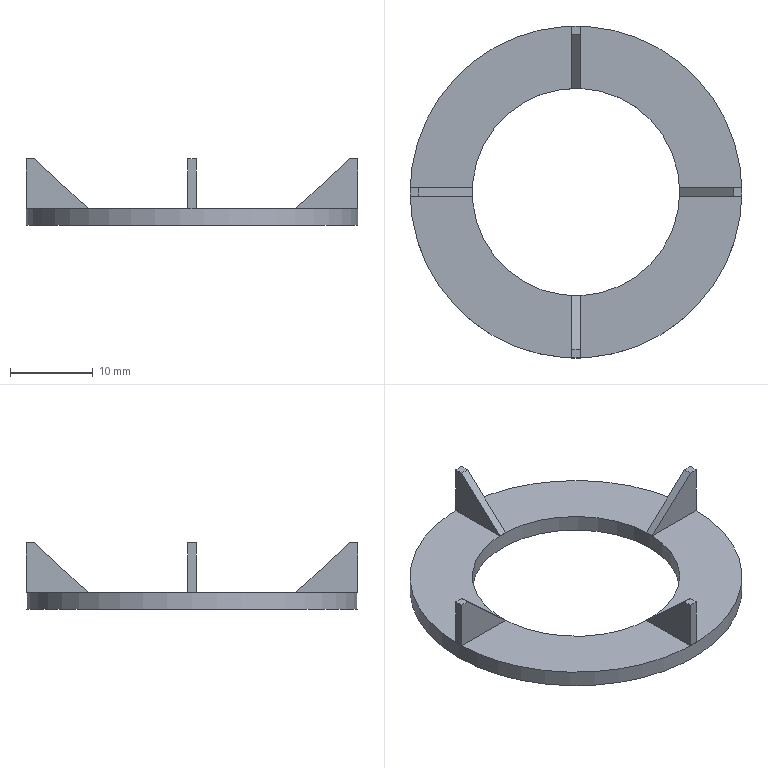Part | NX | features EXTRUDE 5, EXTRACT_STRING 4, DATUM_CSYS 3, Instance Feature 3, SKETCH 2, Pattern Feature 1 | 5 solids | 28 faces | box 40 x 40 x 8 mm | volume 1634 mm3 | plane 26 | cylinder 2 | commonest cylinder face diameters 25 x1 40 x1
STEP:
#1=CARTESIAN_POINT('',(20.,-0.5,8.));
#2=VERTEX_POINT('',#1);
#3=CARTESIAN_POINT('',(20.,-0.5,2.));
#4=VERTEX_POINT('',#3);
#5=CARTESIAN_POINT('',(20.,-0.5,8.));
#6=DIRECTION('',(0.,0.,-1.));
#7=VECTOR('',#6,1000.);
#8=LINE('',#5,#7);
#9=EDGE_CURVE('',#2,#4,#8,.T.);
#10=ORIENTED_EDGE('',*,*,#9,.T.);
#11=CARTESIAN_POINT('',(20.,0.5,2.));
#12=VERTEX_POINT('',#11);
#13=CARTESIAN_POINT('',(20.,0.5,2.));
#14=DIRECTION('',(0.,-1.,0.));
#15=VECTOR('',#14,1000.);
#16=LINE('',#13,#15);
#17=EDGE_CURVE('',#12,#4,#16,.T.);
#18=ORIENTED_EDGE('',*,*,#17,.F.);
#19=CARTESIAN_POINT('',(20.,0.5,8.));
#20=VERTEX_POINT('',#19);
#21=CARTESIAN_POINT('',(20.,0.5,8.));
#22=DIRECTION('',(0.,0.,-1.));
#23=VECTOR('',#22,1000.);
#24=LINE('',#21,#23);
#25=EDGE_CURVE('',#20,#12,#24,.T.);
#26=ORIENTED_EDGE('',*,*,#25,.F.);
#27=CARTESIAN_POINT('',(20.,0.5,8.));
#28=DIRECTION('',(0.,-1.,0.));
#29=VECTOR('',#28,1000.);
#30=LINE('',#27,#29);
#31=EDGE_CURVE('',#20,#2,#30,.T.);
#32=ORIENTED_EDGE('',*,*,#31,.T.);
#33=EDGE_LOOP('',(#10,#18,#26,#32));
#34=FACE_BOUND('',#33,.T.);
#35=CARTESIAN_POINT('',(20.,0.5,8.));
#36=DIRECTION('',(-1.,0.,0.));
#37=DIRECTION('',(0.,-1.,0.));
#38=AXIS2_PLACEMENT_3D('',#35,#36,#37);
#39=PLANE('',#38);
#40=ADVANCED_FACE('',(#34),#39,.F.);
#41=CARTESIAN_POINT('',(12.5,-0.5,2.));
#42=VERTEX_POINT('',#41);
#43=CARTESIAN_POINT('',(20.,-0.5,2.));
#44=DIRECTION('',(-1.,0.,0.));
#45=VECTOR('',#44,1000.);
#46=LINE('',#43,#45);
#47=EDGE_CURVE('',#4,#42,#46,.T.);
#48=ORIENTED_EDGE('',*,*,#47,.T.);
#49=CARTESIAN_POINT('',(12.5,0.5,2.));
#50=VERTEX_POINT('',#49);
#51=CARTESIAN_POINT('',(12.5,0.5,2.));
#52=DIRECTION('',(0.,-1.,0.));
#53=VECTOR('',#52,1000.);
#54=LINE('',#51,#53);
#55=EDGE_CURVE('',#50,#42,#54,.T.);
#56=ORIENTED_EDGE('',*,*,#55,.F.);
#57=CARTESIAN_POINT('',(20.,0.5,2.));
#58=DIRECTION('',(-1.,0.,0.));
#59=VECTOR('',#58,1000.);
#60=LINE('',#57,#59);
#61=EDGE_CURVE('',#12,#50,#60,.T.);
#62=ORIENTED_EDGE('',*,*,#61,.F.);
#63=ORIENTED_EDGE('',*,*,#17,.T.);
#64=EDGE_LOOP('',(#48,#56,#62,#63));
#65=FACE_BOUND('',#64,.T.);
#66=CARTESIAN_POINT('',(20.,0.5,2.));
#67=DIRECTION('',(0.,0.,1.));
#68=DIRECTION('',(1.,0.,0.));
#69=AXIS2_PLACEMENT_3D('',#66,#67,#68);
#70=PLANE('',#69);
#71=ADVANCED_FACE('',(#65),#70,.F.);
#72=CARTESIAN_POINT('',(19.,-0.5,8.));
#73=VERTEX_POINT('',#72);
#74=CARTESIAN_POINT('',(12.5,-0.5,2.));
#75=DIRECTION('',(0.7348,0.,0.6783));
#76=VECTOR('',#75,1000.);
#77=LINE('',#74,#76);
#78=EDGE_CURVE('',#42,#73,#77,.T.);
#79=ORIENTED_EDGE('',*,*,#78,.T.);
#80=CARTESIAN_POINT('',(19.,0.5,8.));
#81=VERTEX_POINT('',#80);
#82=CARTESIAN_POINT('',(19.,0.5,8.));
#83=DIRECTION('',(0.,-1.,0.));
#84=VECTOR('',#83,1000.);
#85=LINE('',#82,#84);
#86=EDGE_CURVE('',#81,#73,#85,.T.);
#87=ORIENTED_EDGE('',*,*,#86,.F.);
#88=CARTESIAN_POINT('',(12.5,0.5,2.));
#89=DIRECTION('',(0.7348,0.,0.6783));
#90=VECTOR('',#89,1000.);
#91=LINE('',#88,#90);
#92=EDGE_CURVE('',#50,#81,#91,.T.);
#93=ORIENTED_EDGE('',*,*,#92,.F.);
#94=ORIENTED_EDGE('',*,*,#55,.T.);
#95=EDGE_LOOP('',(#79,#87,#93,#94));
#96=FACE_BOUND('',#95,.T.);
#97=CARTESIAN_POINT('',(12.5,0.5,2.));
#98=DIRECTION('',(0.6783,0.,-0.7348));
#99=DIRECTION('',(-0.7348,0.,-0.6783));
#100=AXIS2_PLACEMENT_3D('',#97,#98,#99);
#101=PLANE('',#100);
#102=ADVANCED_FACE('',(#96),#101,.F.);
#103=CARTESIAN_POINT('',(19.,-0.5,8.));
#104=DIRECTION('',(1.,0.,0.));
#105=VECTOR('',#104,1000.);
#106=LINE('',#103,#105);
#107=EDGE_CURVE('',#73,#2,#106,.T.);
#108=ORIENTED_EDGE('',*,*,#107,.T.);
#109=ORIENTED_EDGE('',*,*,#31,.F.);
#110=CARTESIAN_POINT('',(19.,0.5,8.));
#111=DIRECTION('',(1.,0.,0.));
#112=VECTOR('',#111,1000.);
#113=LINE('',#110,#112);
#114=EDGE_CURVE('',#81,#20,#113,.T.);
#115=ORIENTED_EDGE('',*,*,#114,.F.);
#116=ORIENTED_EDGE('',*,*,#86,.T.);
#117=EDGE_LOOP('',(#108,#109,#115,#116));
#118=FACE_BOUND('',#117,.T.);
#119=CARTESIAN_POINT('',(19.,0.5,8.));
#120=DIRECTION('',(0.,0.,-1.));
#121=DIRECTION('',(-1.,0.,0.));
#122=AXIS2_PLACEMENT_3D('',#119,#120,#121);
#123=PLANE('',#122);
#124=ADVANCED_FACE('',(#118),#123,.F.);
#125=ORIENTED_EDGE('',*,*,#25,.T.);
#126=ORIENTED_EDGE('',*,*,#61,.T.);
#127=ORIENTED_EDGE('',*,*,#92,.T.);
#128=ORIENTED_EDGE('',*,*,#114,.T.);
#129=EDGE_LOOP('',(#125,#126,#127,#128));
#130=FACE_BOUND('',#129,.T.);
#131=CARTESIAN_POINT('',(0.,0.5,0.));
#132=DIRECTION('',(0.,1.,0.));
#133=DIRECTION('',(-1.,0.,0.));
#134=AXIS2_PLACEMENT_3D('',#131,#132,#133);
#135=PLANE('',#134);
#136=ADVANCED_FACE('',(#130),#135,.T.);
#137=ORIENTED_EDGE('',*,*,#9,.F.);
#138=ORIENTED_EDGE('',*,*,#107,.F.);
#139=ORIENTED_EDGE('',*,*,#78,.F.);
#140=ORIENTED_EDGE('',*,*,#47,.F.);
#141=EDGE_LOOP('',(#137,#138,#139,#140));
#142=FACE_BOUND('',#141,.T.);
#143=CARTESIAN_POINT('',(0.,-0.5,0.));
#144=DIRECTION('',(0.,1.,0.));
#145=DIRECTION('',(-1.,0.,0.));
#146=AXIS2_PLACEMENT_3D('',#143,#144,#145);
#147=PLANE('',#146);
#148=ADVANCED_FACE('',(#142),#147,.F.);
#149=CLOSED_SHELL('',(#40,#71,#102,#124,#136,#148));
#150=MANIFOLD_SOLID_BREP('',#149);
#151=CARTESIAN_POINT('',(-20.,0.5,8.));
#152=VERTEX_POINT('',#151);
#153=CARTESIAN_POINT('',(-20.,0.5,2.));
#154=VERTEX_POINT('',#153);
#155=CARTESIAN_POINT('',(-20.,0.5,8.));
#156=DIRECTION('',(0.,0.,-1.));
#157=VECTOR('',#156,1000.);
#158=LINE('',#155,#157);
#159=EDGE_CURVE('',#152,#154,#158,.T.);
#160=ORIENTED_EDGE('',*,*,#159,.T.);
#161=CARTESIAN_POINT('',(-20.,-0.5,2.));
#162=VERTEX_POINT('',#161);
#163=CARTESIAN_POINT('',(-20.,-0.5,2.));
#164=DIRECTION('',(0.,1.,0.));
#165=VECTOR('',#164,1000.);
#166=LINE('',#163,#165);
#167=EDGE_CURVE('',#162,#154,#166,.T.);
#168=ORIENTED_EDGE('',*,*,#167,.F.);
#169=CARTESIAN_POINT('',(-20.,-0.5,8.));
#170=VERTEX_POINT('',#169);
#171=CARTESIAN_POINT('',(-20.,-0.5,8.));
#172=DIRECTION('',(0.,0.,-1.));
#173=VECTOR('',#172,1000.);
#174=LINE('',#171,#173);
#175=EDGE_CURVE('',#170,#162,#174,.T.);
#176=ORIENTED_EDGE('',*,*,#175,.F.);
#177=CARTESIAN_POINT('',(-20.,-0.5,8.));
#178=DIRECTION('',(0.,1.,0.));
#179=VECTOR('',#178,1000.);
#180=LINE('',#177,#179);
#181=EDGE_CURVE('',#170,#152,#180,.T.);
#182=ORIENTED_EDGE('',*,*,#181,.T.);
#183=EDGE_LOOP('',(#160,#168,#176,#182));
#184=FACE_BOUND('',#183,.T.);
#185=CARTESIAN_POINT('',(-20.,-0.5,8.));
#186=DIRECTION('',(1.,0.,0.));
#187=DIRECTION('',(0.,1.,0.));
#188=AXIS2_PLACEMENT_3D('',#185,#186,#187);
#189=PLANE('',#188);
#190=ADVANCED_FACE('',(#184),#189,.F.);
#191=CARTESIAN_POINT('',(-12.5,0.5,2.));
#192=VERTEX_POINT('',#191);
#193=CARTESIAN_POINT('',(-20.,0.5,2.));
#194=DIRECTION('',(1.,0.,0.));
#195=VECTOR('',#194,1000.);
#196=LINE('',#193,#195);
#197=EDGE_CURVE('',#154,#192,#196,.T.);
#198=ORIENTED_EDGE('',*,*,#197,.T.);
#199=CARTESIAN_POINT('',(-12.5,-0.5,2.));
#200=VERTEX_POINT('',#199);
#201=CARTESIAN_POINT('',(-12.5,-0.5,2.));
#202=DIRECTION('',(0.,1.,0.));
#203=VECTOR('',#202,1000.);
#204=LINE('',#201,#203);
#205=EDGE_CURVE('',#200,#192,#204,.T.);
#206=ORIENTED_EDGE('',*,*,#205,.F.);
#207=CARTESIAN_POINT('',(-20.,-0.5,2.));
#208=DIRECTION('',(1.,0.,0.));
#209=VECTOR('',#208,1000.);
#210=LINE('',#207,#209);
#211=EDGE_CURVE('',#162,#200,#210,.T.);
#212=ORIENTED_EDGE('',*,*,#211,.F.);
#213=ORIENTED_EDGE('',*,*,#167,.T.);
#214=EDGE_LOOP('',(#198,#206,#212,#213));
#215=FACE_BOUND('',#214,.T.);
#216=CARTESIAN_POINT('',(-20.,-0.5,2.));
#217=DIRECTION('',(0.,0.,1.));
#218=DIRECTION('',(1.,0.,0.));
#219=AXIS2_PLACEMENT_3D('',#216,#217,#218);
#220=PLANE('',#219);
#221=ADVANCED_FACE('',(#215),#220,.F.);
#222=CARTESIAN_POINT('',(-19.,0.5,8.));
#223=VERTEX_POINT('',#222);
#224=CARTESIAN_POINT('',(-12.5,0.5,2.));
#225=DIRECTION('',(-0.7348,0.,0.6783));
#226=VECTOR('',#225,1000.);
#227=LINE('',#224,#226);
#228=EDGE_CURVE('',#192,#223,#227,.T.);
#229=ORIENTED_EDGE('',*,*,#228,.T.);
#230=CARTESIAN_POINT('',(-19.,-0.5,8.));
#231=VERTEX_POINT('',#230);
#232=CARTESIAN_POINT('',(-19.,-0.5,8.));
#233=DIRECTION('',(0.,1.,0.));
#234=VECTOR('',#233,1000.);
#235=LINE('',#232,#234);
#236=EDGE_CURVE('',#231,#223,#235,.T.);
#237=ORIENTED_EDGE('',*,*,#236,.F.);
#238=CARTESIAN_POINT('',(-12.5,-0.5,2.));
#239=DIRECTION('',(-0.7348,0.,0.6783));
#240=VECTOR('',#239,1000.);
#241=LINE('',#238,#240);
#242=EDGE_CURVE('',#200,#231,#241,.T.);
#243=ORIENTED_EDGE('',*,*,#242,.F.);
#244=ORIENTED_EDGE('',*,*,#205,.T.);
#245=EDGE_LOOP('',(#229,#237,#243,#244));
#246=FACE_BOUND('',#245,.T.);
#247=CARTESIAN_POINT('',(-12.5,-0.5,2.));
#248=DIRECTION('',(-0.6783,0.,-0.7348));
#249=DIRECTION('',(-0.7348,0.,0.6783));
#250=AXIS2_PLACEMENT_3D('',#247,#248,#249);
#251=PLANE('',#250);
#252=ADVANCED_FACE('',(#246),#251,.F.);
#253=CARTESIAN_POINT('',(-19.,0.5,8.));
#254=DIRECTION('',(-1.,0.,0.));
#255=VECTOR('',#254,1000.);
#256=LINE('',#253,#255);
#257=EDGE_CURVE('',#223,#152,#256,.T.);
#258=ORIENTED_EDGE('',*,*,#257,.T.);
#259=ORIENTED_EDGE('',*,*,#181,.F.);
#260=CARTESIAN_POINT('',(-19.,-0.5,8.));
#261=DIRECTION('',(-1.,0.,0.));
#262=VECTOR('',#261,1000.);
#263=LINE('',#260,#262);
#264=EDGE_CURVE('',#231,#170,#263,.T.);
#265=ORIENTED_EDGE('',*,*,#264,.F.);
#266=ORIENTED_EDGE('',*,*,#236,.T.);
#267=EDGE_LOOP('',(#258,#259,#265,#266));
#268=FACE_BOUND('',#267,.T.);
#269=CARTESIAN_POINT('',(-19.,-0.5,8.));
#270=DIRECTION('',(0.,0.,-1.));
#271=DIRECTION('',(-1.,0.,0.));
#272=AXIS2_PLACEMENT_3D('',#269,#270,#271);
#273=PLANE('',#272);
#274=ADVANCED_FACE('',(#268),#273,.F.);
#275=ORIENTED_EDGE('',*,*,#175,.T.);
#276=ORIENTED_EDGE('',*,*,#211,.T.);
#277=ORIENTED_EDGE('',*,*,#242,.T.);
#278=ORIENTED_EDGE('',*,*,#264,.T.);
#279=EDGE_LOOP('',(#275,#276,#277,#278));
#280=FACE_BOUND('',#279,.T.);
#281=CARTESIAN_POINT('',(0.,-0.5,0.));
#282=DIRECTION('',(0.,-1.,0.));
#283=DIRECTION('',(1.,0.,0.));
#284=AXIS2_PLACEMENT_3D('',#281,#282,#283);
#285=PLANE('',#284);
#286=ADVANCED_FACE('',(#280),#285,.T.);
#287=ORIENTED_EDGE('',*,*,#159,.F.);
#288=ORIENTED_EDGE('',*,*,#257,.F.);
#289=ORIENTED_EDGE('',*,*,#228,.F.);
#290=ORIENTED_EDGE('',*,*,#197,.F.);
#291=EDGE_LOOP('',(#287,#288,#289,#290));
#292=FACE_BOUND('',#291,.T.);
#293=CARTESIAN_POINT('',(0.,0.5,0.));
#294=DIRECTION('',(0.,-1.,0.));
#295=DIRECTION('',(1.,0.,0.));
#296=AXIS2_PLACEMENT_3D('',#293,#294,#295);
#297=PLANE('',#296);
#298=ADVANCED_FACE('',(#292),#297,.F.);
#299=CLOSED_SHELL('',(#190,#221,#252,#274,#286,#298));
#300=MANIFOLD_SOLID_BREP('',#299);
#301=CARTESIAN_POINT('',(20.,0.,0.));
#302=VERTEX_POINT('',#301);
#303=CARTESIAN_POINT('',(0.,0.,0.));
#304=DIRECTION('',(0.,0.,1.));
#305=DIRECTION('',(1.,0.,0.));
#306=AXIS2_PLACEMENT_3D('',#303,#304,#305);
#307=CIRCLE('',#306,20.);
#308=EDGE_CURVE('',#302,#302,#307,.T.);
#309=ORIENTED_EDGE('',*,*,#308,.T.);
#310=EDGE_LOOP('',(#309));
#311=FACE_BOUND('',#310,.T.);
#312=CARTESIAN_POINT('',(20.,0.,2.));
#313=VERTEX_POINT('',#312);
#314=CARTESIAN_POINT('',(0.,0.,2.));
#315=DIRECTION('',(0.,0.,1.));
#316=DIRECTION('',(1.,0.,0.));
#317=AXIS2_PLACEMENT_3D('',#314,#315,#316);
#318=CIRCLE('',#317,20.);
#319=EDGE_CURVE('',#313,#313,#318,.T.);
#320=ORIENTED_EDGE('',*,*,#319,.F.);
#321=EDGE_LOOP('',(#320));
#322=FACE_BOUND('',#321,.T.);
#323=CARTESIAN_POINT('',(0.,0.,0.));
#324=DIRECTION('',(0.,0.,1.));
#325=DIRECTION('',(1.,0.,0.));
#326=AXIS2_PLACEMENT_3D('',#323,#324,#325);
#327=CYLINDRICAL_SURFACE('',#326,20.);
#328=ADVANCED_FACE('',(#311,#322),#327,.T.);
#329=CARTESIAN_POINT('',(12.5,0.,0.));
#330=VERTEX_POINT('',#329);
#331=CARTESIAN_POINT('',(0.,0.,0.));
#332=DIRECTION('',(0.,0.,1.));
#333=DIRECTION('',(1.,0.,0.));
#334=AXIS2_PLACEMENT_3D('',#331,#332,#333);
#335=CIRCLE('',#334,12.5);
#336=EDGE_CURVE('',#330,#330,#335,.T.);
#337=ORIENTED_EDGE('',*,*,#336,.F.);
#338=EDGE_LOOP('',(#337));
#339=FACE_BOUND('',#338,.T.);
#340=CARTESIAN_POINT('',(12.5,0.,2.));
#341=VERTEX_POINT('',#340);
#342=CARTESIAN_POINT('',(0.,0.,2.));
#343=DIRECTION('',(0.,0.,1.));
#344=DIRECTION('',(1.,0.,0.));
#345=AXIS2_PLACEMENT_3D('',#342,#343,#344);
#346=CIRCLE('',#345,12.5);
#347=EDGE_CURVE('',#341,#341,#346,.T.);
#348=ORIENTED_EDGE('',*,*,#347,.T.);
#349=EDGE_LOOP('',(#348));
#350=FACE_BOUND('',#349,.T.);
#351=CARTESIAN_POINT('',(0.,0.,0.));
#352=DIRECTION('',(0.,0.,1.));
#353=DIRECTION('',(1.,0.,0.));
#354=AXIS2_PLACEMENT_3D('',#351,#352,#353);
#355=CYLINDRICAL_SURFACE('',#354,12.5);
#356=ADVANCED_FACE('',(#339,#350),#355,.F.);
#357=ORIENTED_EDGE('',*,*,#308,.F.);
#358=EDGE_LOOP('',(#357));
#359=FACE_BOUND('',#358,.T.);
#360=ORIENTED_EDGE('',*,*,#336,.T.);
#361=EDGE_LOOP('',(#360));
#362=FACE_BOUND('',#361,.T.);
#363=CARTESIAN_POINT('',(0.,0.,0.));
#364=DIRECTION('',(0.,0.,1.));
#365=DIRECTION('',(1.,0.,0.));
#366=AXIS2_PLACEMENT_3D('',#363,#364,#365);
#367=PLANE('',#366);
#368=ADVANCED_FACE('',(#359,#362),#367,.F.);
#369=ORIENTED_EDGE('',*,*,#319,.T.);
#370=EDGE_LOOP('',(#369));
#371=FACE_BOUND('',#370,.T.);
#372=ORIENTED_EDGE('',*,*,#347,.F.);
#373=EDGE_LOOP('',(#372));
#374=FACE_BOUND('',#373,.T.);
#375=CARTESIAN_POINT('',(0.,0.,2.));
#376=DIRECTION('',(0.,0.,1.));
#377=DIRECTION('',(1.,0.,0.));
#378=AXIS2_PLACEMENT_3D('',#375,#376,#377);
#379=PLANE('',#378);
#380=ADVANCED_FACE('',(#371,#374),#379,.T.);
#381=CLOSED_SHELL('',(#328,#356,#368,#380));
#382=MANIFOLD_SOLID_BREP('',#381);
#383=CARTESIAN_POINT('',(0.5,20.,8.));
#384=VERTEX_POINT('',#383);
#385=CARTESIAN_POINT('',(0.5,20.,2.));
#386=VERTEX_POINT('',#385);
#387=CARTESIAN_POINT('',(0.5,20.,8.));
#388=DIRECTION('',(0.,0.,-1.));
#389=VECTOR('',#388,1000.);
#390=LINE('',#387,#389);
#391=EDGE_CURVE('',#384,#386,#390,.T.);
#392=ORIENTED_EDGE('',*,*,#391,.T.);
#393=CARTESIAN_POINT('',(-0.5,20.,2.));
#394=VERTEX_POINT('',#393);
#395=CARTESIAN_POINT('',(-0.5,20.,2.));
#396=DIRECTION('',(1.,0.,0.));
#397=VECTOR('',#396,1000.);
#398=LINE('',#395,#397);
#399=EDGE_CURVE('',#394,#386,#398,.T.);
#400=ORIENTED_EDGE('',*,*,#399,.F.);
#401=CARTESIAN_POINT('',(-0.5,20.,8.));
#402=VERTEX_POINT('',#401);
#403=CARTESIAN_POINT('',(-0.5,20.,8.));
#404=DIRECTION('',(0.,0.,-1.));
#405=VECTOR('',#404,1000.);
#406=LINE('',#403,#405);
#407=EDGE_CURVE('',#402,#394,#406,.T.);
#408=ORIENTED_EDGE('',*,*,#407,.F.);
#409=CARTESIAN_POINT('',(-0.5,20.,8.));
#410=DIRECTION('',(1.,0.,0.));
#411=VECTOR('',#410,1000.);
#412=LINE('',#409,#411);
#413=EDGE_CURVE('',#402,#384,#412,.T.);
#414=ORIENTED_EDGE('',*,*,#413,.T.);
#415=EDGE_LOOP('',(#392,#400,#408,#414));
#416=FACE_BOUND('',#415,.T.);
#417=CARTESIAN_POINT('',(-0.5,20.,8.));
#418=DIRECTION('',(0.,-1.,0.));
#419=DIRECTION('',(1.,0.,0.));
#420=AXIS2_PLACEMENT_3D('',#417,#418,#419);
#421=PLANE('',#420);
#422=ADVANCED_FACE('',(#416),#421,.F.);
#423=CARTESIAN_POINT('',(0.5,12.5,2.));
#424=VERTEX_POINT('',#423);
#425=CARTESIAN_POINT('',(0.5,20.,2.));
#426=DIRECTION('',(0.,-1.,0.));
#427=VECTOR('',#426,1000.);
#428=LINE('',#425,#427);
#429=EDGE_CURVE('',#386,#424,#428,.T.);
#430=ORIENTED_EDGE('',*,*,#429,.T.);
#431=CARTESIAN_POINT('',(-0.5,12.5,2.));
#432=VERTEX_POINT('',#431);
#433=CARTESIAN_POINT('',(-0.5,12.5,2.));
#434=DIRECTION('',(1.,0.,0.));
#435=VECTOR('',#434,1000.);
#436=LINE('',#433,#435);
#437=EDGE_CURVE('',#432,#424,#436,.T.);
#438=ORIENTED_EDGE('',*,*,#437,.F.);
#439=CARTESIAN_POINT('',(-0.5,20.,2.));
#440=DIRECTION('',(0.,-1.,0.));
#441=VECTOR('',#440,1000.);
#442=LINE('',#439,#441);
#443=EDGE_CURVE('',#394,#432,#442,.T.);
#444=ORIENTED_EDGE('',*,*,#443,.F.);
#445=ORIENTED_EDGE('',*,*,#399,.T.);
#446=EDGE_LOOP('',(#430,#438,#444,#445));
#447=FACE_BOUND('',#446,.T.);
#448=CARTESIAN_POINT('',(-0.5,20.,2.));
#449=DIRECTION('',(0.,0.,1.));
#450=DIRECTION('',(1.,0.,0.));
#451=AXIS2_PLACEMENT_3D('',#448,#449,#450);
#452=PLANE('',#451);
#453=ADVANCED_FACE('',(#447),#452,.F.);
#454=CARTESIAN_POINT('',(0.5,19.,8.));
#455=VERTEX_POINT('',#454);
#456=CARTESIAN_POINT('',(0.5,12.5,2.));
#457=DIRECTION('',(0.,0.7348,0.6783));
#458=VECTOR('',#457,1000.);
#459=LINE('',#456,#458);
#460=EDGE_CURVE('',#424,#455,#459,.T.);
#461=ORIENTED_EDGE('',*,*,#460,.T.);
#462=CARTESIAN_POINT('',(-0.5,19.,8.));
#463=VERTEX_POINT('',#462);
#464=CARTESIAN_POINT('',(-0.5,19.,8.));
#465=DIRECTION('',(1.,0.,0.));
#466=VECTOR('',#465,1000.);
#467=LINE('',#464,#466);
#468=EDGE_CURVE('',#463,#455,#467,.T.);
#469=ORIENTED_EDGE('',*,*,#468,.F.);
#470=CARTESIAN_POINT('',(-0.5,12.5,2.));
#471=DIRECTION('',(0.,0.7348,0.6783));
#472=VECTOR('',#471,1000.);
#473=LINE('',#470,#472);
#474=EDGE_CURVE('',#432,#463,#473,.T.);
#475=ORIENTED_EDGE('',*,*,#474,.F.);
#476=ORIENTED_EDGE('',*,*,#437,.T.);
#477=EDGE_LOOP('',(#461,#469,#475,#476));
#478=FACE_BOUND('',#477,.T.);
#479=CARTESIAN_POINT('',(-0.5,12.5,2.));
#480=DIRECTION('',(0.,0.6783,-0.7348));
#481=DIRECTION('',(0.,0.7348,0.6783));
#482=AXIS2_PLACEMENT_3D('',#479,#480,#481);
#483=PLANE('',#482);
#484=ADVANCED_FACE('',(#478),#483,.F.);
#485=CARTESIAN_POINT('',(0.5,19.,8.));
#486=DIRECTION('',(0.,1.,0.));
#487=VECTOR('',#486,1000.);
#488=LINE('',#485,#487);
#489=EDGE_CURVE('',#455,#384,#488,.T.);
#490=ORIENTED_EDGE('',*,*,#489,.T.);
#491=ORIENTED_EDGE('',*,*,#413,.F.);
#492=CARTESIAN_POINT('',(-0.5,19.,8.));
#493=DIRECTION('',(0.,1.,0.));
#494=VECTOR('',#493,1000.);
#495=LINE('',#492,#494);
#496=EDGE_CURVE('',#463,#402,#495,.T.);
#497=ORIENTED_EDGE('',*,*,#496,.F.);
#498=ORIENTED_EDGE('',*,*,#468,.T.);
#499=EDGE_LOOP('',(#490,#491,#497,#498));
#500=FACE_BOUND('',#499,.T.);
#501=CARTESIAN_POINT('',(-0.5,19.,8.));
#502=DIRECTION('',(0.,0.,-1.));
#503=DIRECTION('',(-1.,0.,0.));
#504=AXIS2_PLACEMENT_3D('',#501,#502,#503);
#505=PLANE('',#504);
#506=ADVANCED_FACE('',(#500),#505,.F.);
#507=ORIENTED_EDGE('',*,*,#407,.T.);
#508=ORIENTED_EDGE('',*,*,#443,.T.);
#509=ORIENTED_EDGE('',*,*,#474,.T.);
#510=ORIENTED_EDGE('',*,*,#496,.T.);
#511=EDGE_LOOP('',(#507,#508,#509,#510));
#512=FACE_BOUND('',#511,.T.);
#513=CARTESIAN_POINT('',(-0.5,0.,0.));
#514=DIRECTION('',(-1.,0.,0.));
#515=DIRECTION('',(0.,-1.,0.));
#516=AXIS2_PLACEMENT_3D('',#513,#514,#515);
#517=PLANE('',#516);
#518=ADVANCED_FACE('',(#512),#517,.T.);
#519=ORIENTED_EDGE('',*,*,#391,.F.);
#520=ORIENTED_EDGE('',*,*,#489,.F.);
#521=ORIENTED_EDGE('',*,*,#460,.F.);
#522=ORIENTED_EDGE('',*,*,#429,.F.);
#523=EDGE_LOOP('',(#519,#520,#521,#522));
#524=FACE_BOUND('',#523,.T.);
#525=CARTESIAN_POINT('',(0.5,0.,0.));
#526=DIRECTION('',(-1.,0.,0.));
#527=DIRECTION('',(0.,-1.,0.));
#528=AXIS2_PLACEMENT_3D('',#525,#526,#527);
#529=PLANE('',#528);
#530=ADVANCED_FACE('',(#524),#529,.F.);
#531=CLOSED_SHELL('',(#422,#453,#484,#506,#518,#530));
#532=MANIFOLD_SOLID_BREP('',#531);
#533=CARTESIAN_POINT('',(-0.5,-20.,8.));
#534=VERTEX_POINT('',#533);
#535=CARTESIAN_POINT('',(-0.5,-20.,2.));
#536=VERTEX_POINT('',#535);
#537=CARTESIAN_POINT('',(-0.5,-20.,8.));
#538=DIRECTION('',(0.,0.,-1.));
#539=VECTOR('',#538,1000.);
#540=LINE('',#537,#539);
#541=EDGE_CURVE('',#534,#536,#540,.T.);
#542=ORIENTED_EDGE('',*,*,#541,.T.);
#543=CARTESIAN_POINT('',(0.5,-20.,2.));
#544=VERTEX_POINT('',#543);
#545=CARTESIAN_POINT('',(0.5,-20.,2.));
#546=DIRECTION('',(-1.,0.,0.));
#547=VECTOR('',#546,1000.);
#548=LINE('',#545,#547);
#549=EDGE_CURVE('',#544,#536,#548,.T.);
#550=ORIENTED_EDGE('',*,*,#549,.F.);
#551=CARTESIAN_POINT('',(0.5,-20.,8.));
#552=VERTEX_POINT('',#551);
#553=CARTESIAN_POINT('',(0.5,-20.,8.));
#554=DIRECTION('',(0.,0.,-1.));
#555=VECTOR('',#554,1000.);
#556=LINE('',#553,#555);
#557=EDGE_CURVE('',#552,#544,#556,.T.);
#558=ORIENTED_EDGE('',*,*,#557,.F.);
#559=CARTESIAN_POINT('',(0.5,-20.,8.));
#560=DIRECTION('',(-1.,0.,0.));
#561=VECTOR('',#560,1000.);
#562=LINE('',#559,#561);
#563=EDGE_CURVE('',#552,#534,#562,.T.);
#564=ORIENTED_EDGE('',*,*,#563,.T.);
#565=EDGE_LOOP('',(#542,#550,#558,#564));
#566=FACE_BOUND('',#565,.T.);
#567=CARTESIAN_POINT('',(0.5,-20.,8.));
#568=DIRECTION('',(0.,1.,0.));
#569=DIRECTION('',(0.,0.,1.));
#570=AXIS2_PLACEMENT_3D('',#567,#568,#569);
#571=PLANE('',#570);
#572=ADVANCED_FACE('',(#566),#571,.F.);
#573=CARTESIAN_POINT('',(-0.5,-12.5,2.));
#574=VERTEX_POINT('',#573);
#575=CARTESIAN_POINT('',(-0.5,-20.,2.));
#576=DIRECTION('',(0.,1.,0.));
#577=VECTOR('',#576,1000.);
#578=LINE('',#575,#577);
#579=EDGE_CURVE('',#536,#574,#578,.T.);
#580=ORIENTED_EDGE('',*,*,#579,.T.);
#581=CARTESIAN_POINT('',(0.5,-12.5,2.));
#582=VERTEX_POINT('',#581);
#583=CARTESIAN_POINT('',(0.5,-12.5,2.));
#584=DIRECTION('',(-1.,0.,0.));
#585=VECTOR('',#584,1000.);
#586=LINE('',#583,#585);
#587=EDGE_CURVE('',#582,#574,#586,.T.);
#588=ORIENTED_EDGE('',*,*,#587,.F.);
#589=CARTESIAN_POINT('',(0.5,-20.,2.));
#590=DIRECTION('',(0.,1.,0.));
#591=VECTOR('',#590,1000.);
#592=LINE('',#589,#591);
#593=EDGE_CURVE('',#544,#582,#592,.T.);
#594=ORIENTED_EDGE('',*,*,#593,.F.);
#595=ORIENTED_EDGE('',*,*,#549,.T.);
#596=EDGE_LOOP('',(#580,#588,#594,#595));
#597=FACE_BOUND('',#596,.T.);
#598=CARTESIAN_POINT('',(0.5,-20.,2.));
#599=DIRECTION('',(0.,0.,1.));
#600=DIRECTION('',(1.,0.,0.));
#601=AXIS2_PLACEMENT_3D('',#598,#599,#600);
#602=PLANE('',#601);
#603=ADVANCED_FACE('',(#597),#602,.F.);
#604=CARTESIAN_POINT('',(-0.5,-19.,8.));
#605=VERTEX_POINT('',#604);
#606=CARTESIAN_POINT('',(-0.5,-12.5,2.));
#607=DIRECTION('',(0.,-0.7348,0.6783));
#608=VECTOR('',#607,1000.);
#609=LINE('',#606,#608);
#610=EDGE_CURVE('',#574,#605,#609,.T.);
#611=ORIENTED_EDGE('',*,*,#610,.T.);
#612=CARTESIAN_POINT('',(0.5,-19.,8.));
#613=VERTEX_POINT('',#612);
#614=CARTESIAN_POINT('',(0.5,-19.,8.));
#615=DIRECTION('',(-1.,0.,0.));
#616=VECTOR('',#615,1000.);
#617=LINE('',#614,#616);
#618=EDGE_CURVE('',#613,#605,#617,.T.);
#619=ORIENTED_EDGE('',*,*,#618,.F.);
#620=CARTESIAN_POINT('',(0.5,-12.5,2.));
#621=DIRECTION('',(0.,-0.7348,0.6783));
#622=VECTOR('',#621,1000.);
#623=LINE('',#620,#622);
#624=EDGE_CURVE('',#582,#613,#623,.T.);
#625=ORIENTED_EDGE('',*,*,#624,.F.);
#626=ORIENTED_EDGE('',*,*,#587,.T.);
#627=EDGE_LOOP('',(#611,#619,#625,#626));
#628=FACE_BOUND('',#627,.T.);
#629=CARTESIAN_POINT('',(0.5,-12.5,2.));
#630=DIRECTION('',(0.,-0.6783,-0.7348));
#631=DIRECTION('',(0.,0.7348,-0.6783));
#632=AXIS2_PLACEMENT_3D('',#629,#630,#631);
#633=PLANE('',#632);
#634=ADVANCED_FACE('',(#628),#633,.F.);
#635=CARTESIAN_POINT('',(-0.5,-19.,8.));
#636=DIRECTION('',(0.,-1.,0.));
#637=VECTOR('',#636,1000.);
#638=LINE('',#635,#637);
#639=EDGE_CURVE('',#605,#534,#638,.T.);
#640=ORIENTED_EDGE('',*,*,#639,.T.);
#641=ORIENTED_EDGE('',*,*,#563,.F.);
#642=CARTESIAN_POINT('',(0.5,-19.,8.));
#643=DIRECTION('',(0.,-1.,0.));
#644=VECTOR('',#643,1000.);
#645=LINE('',#642,#644);
#646=EDGE_CURVE('',#613,#552,#645,.T.);
#647=ORIENTED_EDGE('',*,*,#646,.F.);
#648=ORIENTED_EDGE('',*,*,#618,.T.);
#649=EDGE_LOOP('',(#640,#641,#647,#648));
#650=FACE_BOUND('',#649,.T.);
#651=CARTESIAN_POINT('',(0.5,-19.,8.));
#652=DIRECTION('',(0.,0.,-1.));
#653=DIRECTION('',(-1.,0.,0.));
#654=AXIS2_PLACEMENT_3D('',#651,#652,#653);
#655=PLANE('',#654);
#656=ADVANCED_FACE('',(#650),#655,.F.);
#657=ORIENTED_EDGE('',*,*,#557,.T.);
#658=ORIENTED_EDGE('',*,*,#593,.T.);
#659=ORIENTED_EDGE('',*,*,#624,.T.);
#660=ORIENTED_EDGE('',*,*,#646,.T.);
#661=EDGE_LOOP('',(#657,#658,#659,#660));
#662=FACE_BOUND('',#661,.T.);
#663=CARTESIAN_POINT('',(0.5,0.,0.));
#664=DIRECTION('',(1.,0.,0.));
#665=DIRECTION('',(0.,0.,-1.));
#666=AXIS2_PLACEMENT_3D('',#663,#664,#665);
#667=PLANE('',#666);
#668=ADVANCED_FACE('',(#662),#667,.T.);
#669=ORIENTED_EDGE('',*,*,#541,.F.);
#670=ORIENTED_EDGE('',*,*,#639,.F.);
#671=ORIENTED_EDGE('',*,*,#610,.F.);
#672=ORIENTED_EDGE('',*,*,#579,.F.);
#673=EDGE_LOOP('',(#669,#670,#671,#672));
#674=FACE_BOUND('',#673,.T.);
#675=CARTESIAN_POINT('',(-0.5,0.,0.));
#676=DIRECTION('',(1.,0.,0.));
#677=DIRECTION('',(0.,0.,-1.));
#678=AXIS2_PLACEMENT_3D('',#675,#676,#677);
#679=PLANE('',#678);
#680=ADVANCED_FACE('',(#674),#679,.F.);
#681=CLOSED_SHELL('',(#572,#603,#634,#656,#668,#680));
#682=MANIFOLD_SOLID_BREP('',#681);
#683=(LENGTH_UNIT()NAMED_UNIT(*)SI_UNIT(.MILLI.,.METRE.));
#684=UNCERTAINTY_MEASURE_WITH_UNIT(LENGTH_MEASURE(0.00001),#683,'','');
#685=(NAMED_UNIT(*)PLANE_ANGLE_UNIT()SI_UNIT($,.RADIAN.));
#686=(NAMED_UNIT(*)SI_UNIT($,.STERADIAN.)SOLID_ANGLE_UNIT());
#687=(GEOMETRIC_REPRESENTATION_CONTEXT(3)GLOBAL_UNCERTAINTY_ASSIGNED_CONTEXT((#684))GLOBAL_UNIT_ASSIGNED_CONTEXT((#683,#685,#686))REPRESENTATION_CONTEXT('',''));
#688=ADVANCED_BREP_SHAPE_REPRESENTATION('',(#150,#300,#382,#532,#682),#687);